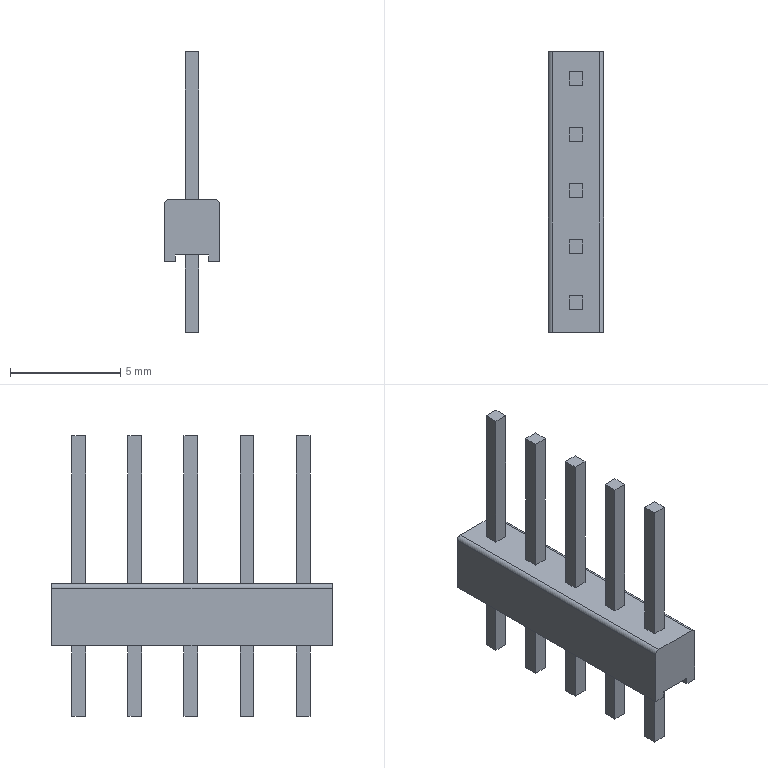Part | STEP file | RJ-USIO-V1_2-220411_249 | 1 solid | 62 faces | box 2.5 x 12.7 x 12.7 mm | volume 103.209 mm3 | plane 60 | cylinder 2 | commonest cylinder face diameters 0.4 x2